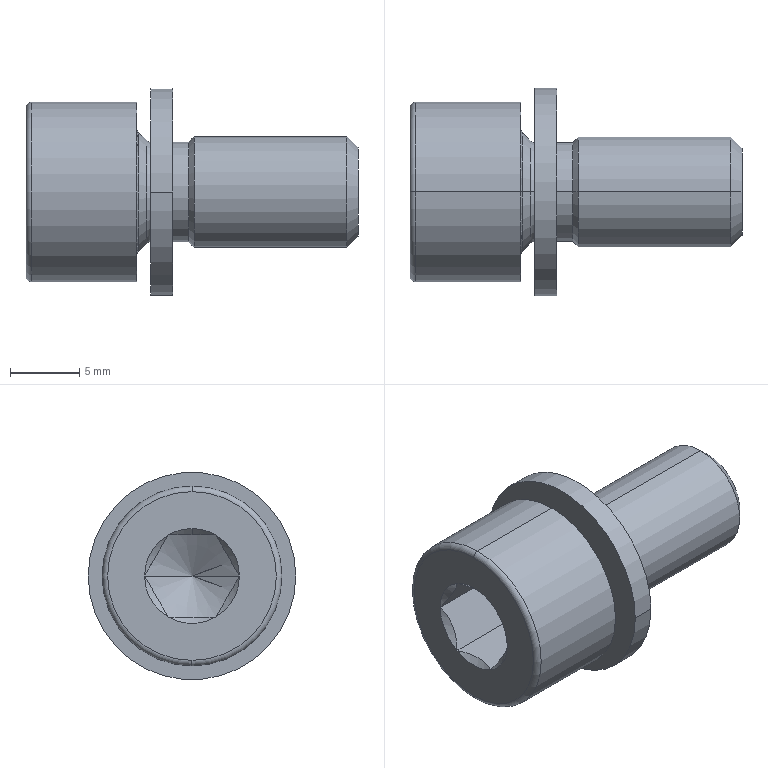Part | SolidWorks | features RevCut 2, Revolution 2, Chamfer 1, Cut 1, Fillet 1 | 2 solids | 48 faces | box 24 x 15 x 15 mm | volume 1870 mm3 | plane 17 | cone 15 | cylinder 10 | torus 6 | commonest cylinder face diameters 7.188 x2 7.55 x2 8 x2 13 x2 15 x2
STEP:
#1=CARTESIAN_POINT('',(10.62,-7.5,0.));
#2=VERTEX_POINT('',#1);
#3=CARTESIAN_POINT('',(10.62,7.5,0.));
#4=VERTEX_POINT('',#3);
#5=CARTESIAN_POINT('',(10.62,0.,0.));
#6=DIRECTION('',(-1.,0.,0.));
#7=DIRECTION('',(0.,-1.,0.));
#8=AXIS2_PLACEMENT_3D('',#5,#6,#7);
#9=CIRCLE('',#8,7.5);
#10=EDGE_CURVE('',#2,#4,#9,.T.);
#11=ORIENTED_EDGE('',*,*,#10,.T.);
#12=CARTESIAN_POINT('',(9.02,7.5,0.));
#13=VERTEX_POINT('',#12);
#14=CARTESIAN_POINT('',(0.,7.5,0.));
#15=DIRECTION('',(-1.,0.,0.));
#16=VECTOR('',#15,1000.);
#17=LINE('',#14,#16);
#18=EDGE_CURVE('',#4,#13,#17,.T.);
#19=ORIENTED_EDGE('',*,*,#18,.T.);
#20=CARTESIAN_POINT('',(9.02,-7.5,0.));
#21=VERTEX_POINT('',#20);
#22=CARTESIAN_POINT('',(9.02,0.,0.));
#23=DIRECTION('',(-1.,0.,0.));
#24=DIRECTION('',(0.,-1.,0.));
#25=AXIS2_PLACEMENT_3D('',#22,#23,#24);
#26=CIRCLE('',#25,7.5);
#27=EDGE_CURVE('',#21,#13,#26,.T.);
#28=ORIENTED_EDGE('',*,*,#27,.F.);
#29=CARTESIAN_POINT('',(0.,-7.5,0.));
#30=DIRECTION('',(-1.,0.,0.));
#31=VECTOR('',#30,1000.);
#32=LINE('',#29,#31);
#33=EDGE_CURVE('',#2,#21,#32,.T.);
#34=ORIENTED_EDGE('',*,*,#33,.F.);
#35=EDGE_LOOP('',(#11,#19,#28,#34));
#36=FACE_OUTER_BOUND('',#35,.T.);
#37=CARTESIAN_POINT('',(0.,0.,0.));
#38=DIRECTION('',(-1.,0.,0.));
#39=DIRECTION('',(0.,-1.,0.));
#40=AXIS2_PLACEMENT_3D('',#37,#38,#39);
#41=CYLINDRICAL_SURFACE('',#40,7.5);
#42=ADVANCED_FACE('',(#36),#41,.T.);
#43=CARTESIAN_POINT('',(10.62,3.775,0.));
#44=VERTEX_POINT('',#43);
#45=CARTESIAN_POINT('',(10.62,-3.775,0.));
#46=VERTEX_POINT('',#45);
#47=CARTESIAN_POINT('',(10.62,0.,0.));
#48=DIRECTION('',(-1.,0.,0.));
#49=DIRECTION('',(0.,-1.,0.));
#50=AXIS2_PLACEMENT_3D('',#47,#48,#49);
#51=CIRCLE('',#50,3.775);
#52=EDGE_CURVE('',#44,#46,#51,.T.);
#53=ORIENTED_EDGE('',*,*,#52,.F.);
#54=CARTESIAN_POINT('',(9.02,3.775,0.));
#55=VERTEX_POINT('',#54);
#56=CARTESIAN_POINT('',(0.,3.775,0.));
#57=DIRECTION('',(-1.,0.,0.));
#58=VECTOR('',#57,1000.);
#59=LINE('',#56,#58);
#60=EDGE_CURVE('',#44,#55,#59,.T.);
#61=ORIENTED_EDGE('',*,*,#60,.T.);
#62=CARTESIAN_POINT('',(9.02,-3.775,0.));
#63=VERTEX_POINT('',#62);
#64=CARTESIAN_POINT('',(9.02,0.,0.));
#65=DIRECTION('',(-1.,0.,0.));
#66=DIRECTION('',(0.,-1.,0.));
#67=AXIS2_PLACEMENT_3D('',#64,#65,#66);
#68=CIRCLE('',#67,3.775);
#69=EDGE_CURVE('',#55,#63,#68,.T.);
#70=ORIENTED_EDGE('',*,*,#69,.T.);
#71=CARTESIAN_POINT('',(0.,-3.775,0.));
#72=DIRECTION('',(-1.,0.,0.));
#73=VECTOR('',#72,1000.);
#74=LINE('',#71,#73);
#75=EDGE_CURVE('',#46,#63,#74,.T.);
#76=ORIENTED_EDGE('',*,*,#75,.F.);
#77=EDGE_LOOP('',(#53,#61,#70,#76));
#78=FACE_OUTER_BOUND('',#77,.T.);
#79=CARTESIAN_POINT('',(0.,0.,0.));
#80=DIRECTION('',(-1.,0.,0.));
#81=DIRECTION('',(0.,-1.,0.));
#82=AXIS2_PLACEMENT_3D('',#79,#80,#81);
#83=CYLINDRICAL_SURFACE('',#82,3.775);
#84=ADVANCED_FACE('',(#78),#83,.F.);
#85=ORIENTED_EDGE('',*,*,#60,.F.);
#86=CARTESIAN_POINT('',(10.62,0.,0.));
#87=DIRECTION('',(-1.,0.,0.));
#88=DIRECTION('',(0.,-1.,0.));
#89=AXIS2_PLACEMENT_3D('',#86,#87,#88);
#90=CIRCLE('',#89,3.775);
#91=EDGE_CURVE('',#46,#44,#90,.T.);
#92=ORIENTED_EDGE('',*,*,#91,.F.);
#93=ORIENTED_EDGE('',*,*,#75,.T.);
#94=CARTESIAN_POINT('',(9.02,0.,0.));
#95=DIRECTION('',(-1.,0.,0.));
#96=DIRECTION('',(0.,-1.,0.));
#97=AXIS2_PLACEMENT_3D('',#94,#95,#96);
#98=CIRCLE('',#97,3.775);
#99=EDGE_CURVE('',#63,#55,#98,.T.);
#100=ORIENTED_EDGE('',*,*,#99,.T.);
#101=EDGE_LOOP('',(#85,#92,#93,#100));
#102=FACE_OUTER_BOUND('',#101,.T.);
#103=CARTESIAN_POINT('',(0.,0.,0.));
#104=DIRECTION('',(-1.,0.,0.));
#105=DIRECTION('',(0.,-1.,0.));
#106=AXIS2_PLACEMENT_3D('',#103,#104,#105);
#107=CYLINDRICAL_SURFACE('',#106,3.775);
#108=ADVANCED_FACE('',(#102),#107,.F.);
#109=ORIENTED_EDGE('',*,*,#99,.F.);
#110=ORIENTED_EDGE('',*,*,#69,.F.);
#111=EDGE_LOOP('',(#109,#110));
#112=FACE_BOUND('',#111,.T.);
#113=ORIENTED_EDGE('',*,*,#27,.T.);
#114=CARTESIAN_POINT('',(9.02,0.,0.));
#115=DIRECTION('',(-1.,0.,0.));
#116=DIRECTION('',(0.,-1.,0.));
#117=AXIS2_PLACEMENT_3D('',#114,#115,#116);
#118=CIRCLE('',#117,7.5);
#119=EDGE_CURVE('',#13,#21,#118,.T.);
#120=ORIENTED_EDGE('',*,*,#119,.T.);
#121=EDGE_LOOP('',(#113,#120));
#122=FACE_OUTER_BOUND('',#121,.T.);
#123=CARTESIAN_POINT('',(9.02,-3.775,0.));
#124=DIRECTION('',(1.,0.,0.));
#125=DIRECTION('',(0.,1.,0.));
#126=AXIS2_PLACEMENT_3D('',#123,#124,#125);
#127=PLANE('',#126);
#128=ADVANCED_FACE('',(#112,#122),#127,.F.);
#129=ORIENTED_EDGE('',*,*,#18,.F.);
#130=CARTESIAN_POINT('',(10.62,0.,0.));
#131=DIRECTION('',(-1.,0.,0.));
#132=DIRECTION('',(0.,-1.,0.));
#133=AXIS2_PLACEMENT_3D('',#130,#131,#132);
#134=CIRCLE('',#133,7.5);
#135=EDGE_CURVE('',#4,#2,#134,.T.);
#136=ORIENTED_EDGE('',*,*,#135,.T.);
#137=ORIENTED_EDGE('',*,*,#33,.T.);
#138=ORIENTED_EDGE('',*,*,#119,.F.);
#139=EDGE_LOOP('',(#129,#136,#137,#138));
#140=FACE_OUTER_BOUND('',#139,.T.);
#141=CARTESIAN_POINT('',(0.,0.,0.));
#142=DIRECTION('',(-1.,0.,0.));
#143=DIRECTION('',(0.,-1.,0.));
#144=AXIS2_PLACEMENT_3D('',#141,#142,#143);
#145=CYLINDRICAL_SURFACE('',#144,7.5);
#146=ADVANCED_FACE('',(#140),#145,.T.);
#147=ORIENTED_EDGE('',*,*,#10,.F.);
#148=ORIENTED_EDGE('',*,*,#135,.F.);
#149=EDGE_LOOP('',(#147,#148));
#150=FACE_OUTER_BOUND('',#149,.T.);
#151=ORIENTED_EDGE('',*,*,#91,.T.);
#152=ORIENTED_EDGE('',*,*,#52,.T.);
#153=EDGE_LOOP('',(#151,#152));
#154=FACE_BOUND('',#153,.T.);
#155=CARTESIAN_POINT('',(10.62,-7.5,0.));
#156=DIRECTION('',(-1.,0.,0.));
#157=DIRECTION('',(0.,-1.,0.));
#158=AXIS2_PLACEMENT_3D('',#155,#156,#157);
#159=PLANE('',#158);
#160=ADVANCED_FACE('',(#150,#154),#159,.F.);
#161=CLOSED_SHELL('',(#42,#84,#108,#128,#146,#160));
#162=MANIFOLD_SOLID_BREP('',#161);
#163=CARTESIAN_POINT('',(24.,0.,-3.2));
#164=VERTEX_POINT('',#163);
#165=CARTESIAN_POINT('',(24.,0.,3.2));
#166=VERTEX_POINT('',#165);
#167=CARTESIAN_POINT('',(24.,0.,0.));
#168=DIRECTION('',(1.,0.,0.));
#169=DIRECTION('',(0.,0.,-1.));
#170=AXIS2_PLACEMENT_3D('',#167,#168,#169);
#171=CIRCLE('',#170,3.2);
#172=EDGE_CURVE('',#164,#166,#171,.T.);
#173=ORIENTED_EDGE('',*,*,#172,.F.);
#174=CARTESIAN_POINT('',(23.2,0.,-4.));
#175=VERTEX_POINT('',#174);
#176=CARTESIAN_POINT('',(24.,0.,-3.2));
#177=DIRECTION('',(-0.7071,0.,-0.7071));
#178=VECTOR('',#177,1000.);
#179=LINE('',#176,#178);
#180=EDGE_CURVE('',#164,#175,#179,.T.);
#181=ORIENTED_EDGE('',*,*,#180,.T.);
#182=CARTESIAN_POINT('',(23.2,0.,4.));
#183=VERTEX_POINT('',#182);
#184=CARTESIAN_POINT('',(23.2,0.,0.));
#185=DIRECTION('',(-1.,0.,0.));
#186=DIRECTION('',(0.,0.,-1.));
#187=AXIS2_PLACEMENT_3D('',#184,#185,#186);
#188=CIRCLE('',#187,4.);
#189=EDGE_CURVE('',#183,#175,#188,.T.);
#190=ORIENTED_EDGE('',*,*,#189,.F.);
#191=CARTESIAN_POINT('',(24.,0.,3.2));
#192=DIRECTION('',(-0.7071,0.,0.7071));
#193=VECTOR('',#192,1000.);
#194=LINE('',#191,#193);
#195=EDGE_CURVE('',#166,#183,#194,.T.);
#196=ORIENTED_EDGE('',*,*,#195,.F.);
#197=EDGE_LOOP('',(#173,#181,#190,#196));
#198=FACE_OUTER_BOUND('',#197,.T.);
#199=CARTESIAN_POINT('',(24.,0.,0.));
#200=DIRECTION('',(-1.,0.,0.));
#201=DIRECTION('',(0.,0.,1.));
#202=AXIS2_PLACEMENT_3D('',#199,#200,#201);
#203=CONICAL_SURFACE('',#202,3.2,0.7854);
#204=ADVANCED_FACE('',(#198),#203,.T.);
#205=CARTESIAN_POINT('',(0.4,0.,-6.5));
#206=VERTEX_POINT('',#205);
#207=CARTESIAN_POINT('',(0.4,0.,6.5));
#208=VERTEX_POINT('',#207);
#209=CARTESIAN_POINT('',(0.4,0.,0.));
#210=DIRECTION('',(1.,0.,0.));
#211=DIRECTION('',(0.,0.,1.));
#212=AXIS2_PLACEMENT_3D('',#209,#210,#211);
#213=CIRCLE('',#212,6.5);
#214=EDGE_CURVE('',#206,#208,#213,.T.);
#215=ORIENTED_EDGE('',*,*,#214,.F.);
#216=CARTESIAN_POINT('',(0.,0.,-6.1));
#217=VERTEX_POINT('',#216);
#218=CARTESIAN_POINT('',(0.4,0.,-6.1));
#219=DIRECTION('',(0.,1.,0.));
#220=DIRECTION('',(0.,0.,1.));
#221=AXIS2_PLACEMENT_3D('',#218,#219,#220);
#222=CIRCLE('',#221,0.4);
#223=EDGE_CURVE('',#206,#217,#222,.T.);
#224=ORIENTED_EDGE('',*,*,#223,.T.);
#225=CARTESIAN_POINT('',(0.,0.,6.1));
#226=VERTEX_POINT('',#225);
#227=CARTESIAN_POINT('',(0.,0.,0.));
#228=DIRECTION('',(-1.,0.,0.));
#229=DIRECTION('',(0.,0.,1.));
#230=AXIS2_PLACEMENT_3D('',#227,#228,#229);
#231=CIRCLE('',#230,6.1);
#232=EDGE_CURVE('',#226,#217,#231,.T.);
#233=ORIENTED_EDGE('',*,*,#232,.F.);
#234=CARTESIAN_POINT('',(0.4,0.,6.1));
#235=DIRECTION('',(0.,-1.,0.));
#236=DIRECTION('',(0.,0.,-1.));
#237=AXIS2_PLACEMENT_3D('',#234,#235,#236);
#238=CIRCLE('',#237,0.4);
#239=EDGE_CURVE('',#208,#226,#238,.T.);
#240=ORIENTED_EDGE('',*,*,#239,.F.);
#241=EDGE_LOOP('',(#215,#224,#233,#240));
#242=FACE_OUTER_BOUND('',#241,.T.);
#243=CARTESIAN_POINT('',(0.4,0.,0.));
#244=DIRECTION('',(-1.,0.,0.));
#245=DIRECTION('',(0.,0.,1.));
#246=AXIS2_PLACEMENT_3D('',#243,#244,#245);
#247=TOROIDAL_SURFACE('',#246,6.1,0.4);
#248=ADVANCED_FACE('',(#242),#247,.T.);
#249=CARTESIAN_POINT('',(6.68,0.,0.));
#250=VERTEX_POINT('',#249);
#251=CARTESIAN_POINT('',(4.7,-3.43,0.));
#252=VERTEX_POINT('',#251);
#253=CARTESIAN_POINT('',(6.68,0.,0.));
#254=DIRECTION('',(-0.5,-0.866,0.));
#255=VECTOR('',#254,1000.);
#256=LINE('',#253,#255);
#257=EDGE_CURVE('',#250,#252,#256,.T.);
#258=ORIENTED_EDGE('',*,*,#257,.F.);
#259=CARTESIAN_POINT('',(4.7,3.43,0.));
#260=VERTEX_POINT('',#259);
#261=CARTESIAN_POINT('',(6.68,0.,0.));
#262=DIRECTION('',(-0.5,0.866,0.));
#263=VECTOR('',#262,1000.);
#264=LINE('',#261,#263);
#265=EDGE_CURVE('',#250,#260,#264,.T.);
#266=ORIENTED_EDGE('',*,*,#265,.T.);
#267=CARTESIAN_POINT('',(4.7,1.715,-2.97));
#268=VERTEX_POINT('',#267);
#269=CARTESIAN_POINT('',(4.7,0.,0.));
#270=DIRECTION('',(-1.,0.,0.));
#271=DIRECTION('',(0.,-1.,0.));
#272=AXIS2_PLACEMENT_3D('',#269,#270,#271);
#273=CIRCLE('',#272,3.43);
#274=EDGE_CURVE('',#260,#268,#273,.T.);
#275=ORIENTED_EDGE('',*,*,#274,.T.);
#276=CARTESIAN_POINT('',(4.7,-1.715,-2.97));
#277=VERTEX_POINT('',#276);
#278=CARTESIAN_POINT('',(4.7,0.,0.));
#279=DIRECTION('',(-1.,0.,0.));
#280=DIRECTION('',(0.,-1.,0.));
#281=AXIS2_PLACEMENT_3D('',#278,#279,#280);
#282=CIRCLE('',#281,3.43);
#283=EDGE_CURVE('',#268,#277,#282,.T.);
#284=ORIENTED_EDGE('',*,*,#283,.T.);
#285=CARTESIAN_POINT('',(4.7,0.,0.));
#286=DIRECTION('',(-1.,0.,0.));
#287=DIRECTION('',(0.,-1.,0.));
#288=AXIS2_PLACEMENT_3D('',#285,#286,#287);
#289=CIRCLE('',#288,3.43);
#290=EDGE_CURVE('',#277,#252,#289,.T.);
#291=ORIENTED_EDGE('',*,*,#290,.T.);
#292=EDGE_LOOP('',(#258,#266,#275,#284,#291));
#293=FACE_OUTER_BOUND('',#292,.T.);
#294=CARTESIAN_POINT('',(-993.32,0.,0.));
#295=DIRECTION('',(-1.,0.,0.));
#296=DIRECTION('',(0.,-1.,0.));
#297=AXIS2_PLACEMENT_3D('',#294,#295,#296);
#298=CONICAL_SURFACE('',#297,1732.051,1.047);
#299=ADVANCED_FACE('',(#293),#298,.F.);
#300=CARTESIAN_POINT('',(0.4595,0.,2.97));
#301=VERTEX_POINT('',#300);
#302=CARTESIAN_POINT('',(0.,1.715,2.97));
#303=VERTEX_POINT('',#302);
#304=CARTESIAN_POINT('',(0.4595,0.,2.97));
#305=CARTESIAN_POINT('',(0.4595,0.3016,2.97));
#306=CARTESIAN_POINT('',(0.4131,0.5952,2.97));
#307=CARTESIAN_POINT('',(0.2902,1.027,2.97));
#308=CARTESIAN_POINT('',(0.2401,1.169,2.97));
#309=CARTESIAN_POINT('',(0.1283,1.447,2.97));
#310=CARTESIAN_POINT('',(0.06637,1.582,2.97));
#311=CARTESIAN_POINT('',(0.,1.715,2.97));
#312=B_SPLINE_CURVE_WITH_KNOTS('',3,(#304,#305,#306,#307,#308,#309,#310,#311),.UNSPECIFIED.,.F.,.F.,(4,2,2,4),(0.004005,0.004894,0.005339,0.005784),.UNSPECIFIED.);
#313=EDGE_CURVE('',#301,#303,#312,.T.);
#314=ORIENTED_EDGE('',*,*,#313,.F.);
#315=CARTESIAN_POINT('',(0.,0.,3.43));
#316=VERTEX_POINT('',#315);
#317=CARTESIAN_POINT('',(0.4595,0.,2.97));
#318=DIRECTION('',(-0.7071,0.,0.7071));
#319=VECTOR('',#318,1000.);
#320=LINE('',#317,#319);
#321=EDGE_CURVE('',#301,#316,#320,.T.);
#322=ORIENTED_EDGE('',*,*,#321,.T.);
#323=CARTESIAN_POINT('',(0.,0.,0.));
#324=DIRECTION('',(1.,0.,0.));
#325=DIRECTION('',(0.,0.,-1.));
#326=AXIS2_PLACEMENT_3D('',#323,#324,#325);
#327=CIRCLE('',#326,3.43);
#328=EDGE_CURVE('',#303,#316,#327,.T.);
#329=ORIENTED_EDGE('',*,*,#328,.F.);
#330=EDGE_LOOP('',(#314,#322,#329));
#331=FACE_OUTER_BOUND('',#330,.T.);
#332=CARTESIAN_POINT('',(0.4595,0.,0.));
#333=DIRECTION('',(-1.,0.,0.));
#334=DIRECTION('',(0.,0.,1.));
#335=AXIS2_PLACEMENT_3D('',#332,#333,#334);
#336=CONICAL_SURFACE('',#335,2.97,0.7854);
#337=ADVANCED_FACE('',(#331),#336,.F.);
#338=CARTESIAN_POINT('',(12.156,0.,-4.));
#339=VERTEX_POINT('',#338);
#340=CARTESIAN_POINT('',(12.156,0.,4.));
#341=VERTEX_POINT('',#340);
#342=CARTESIAN_POINT('',(12.156,0.,0.));
#343=DIRECTION('',(1.,0.,0.));
#344=DIRECTION('',(0.,0.,-1.));
#345=AXIS2_PLACEMENT_3D('',#342,#343,#344);
#346=CIRCLE('',#345,4.);
#347=EDGE_CURVE('',#339,#341,#346,.T.);
#348=ORIENTED_EDGE('',*,*,#347,.T.);
#349=CARTESIAN_POINT('',(0.,0.,4.));
#350=DIRECTION('',(1.,0.,0.));
#351=VECTOR('',#350,1000.);
#352=LINE('',#349,#351);
#353=EDGE_CURVE('',#341,#183,#352,.T.);
#354=ORIENTED_EDGE('',*,*,#353,.T.);
#355=ORIENTED_EDGE('',*,*,#189,.T.);
#356=CARTESIAN_POINT('',(0.,0.,-4.));
#357=DIRECTION('',(1.,0.,0.));
#358=VECTOR('',#357,1000.);
#359=LINE('',#356,#358);
#360=EDGE_CURVE('',#339,#175,#359,.T.);
#361=ORIENTED_EDGE('',*,*,#360,.F.);
#362=EDGE_LOOP('',(#348,#354,#355,#361));
#363=FACE_OUTER_BOUND('',#362,.T.);
#364=CARTESIAN_POINT('',(0.,0.,0.));
#365=DIRECTION('',(1.,0.,0.));
#366=DIRECTION('',(0.,0.,-1.));
#367=AXIS2_PLACEMENT_3D('',#364,#365,#366);
#368=CYLINDRICAL_SURFACE('',#367,4.);
#369=ADVANCED_FACE('',(#363),#368,.T.);
#370=CARTESIAN_POINT('',(11.75,0.,-3.594));
#371=VERTEX_POINT('',#370);
#372=CARTESIAN_POINT('',(11.75,0.,3.594));
#373=VERTEX_POINT('',#372);
#374=CARTESIAN_POINT('',(11.75,0.,0.));
#375=DIRECTION('',(1.,0.,0.));
#376=DIRECTION('',(0.,0.,-1.));
#377=AXIS2_PLACEMENT_3D('',#374,#375,#376);
#378=CIRCLE('',#377,3.594);
#379=EDGE_CURVE('',#371,#373,#378,.T.);
#380=ORIENTED_EDGE('',*,*,#379,.T.);
#381=CARTESIAN_POINT('',(12.156,0.,4.));
#382=DIRECTION('',(0.7071,0.,0.7071));
#383=VECTOR('',#382,1000.);
#384=LINE('',#381,#383);
#385=EDGE_CURVE('',#373,#341,#384,.T.);
#386=ORIENTED_EDGE('',*,*,#385,.T.);
#387=ORIENTED_EDGE('',*,*,#347,.F.);
#388=CARTESIAN_POINT('',(12.156,0.,-4.));
#389=DIRECTION('',(0.7071,0.,-0.7071));
#390=VECTOR('',#389,1000.);
#391=LINE('',#388,#390);
#392=EDGE_CURVE('',#371,#339,#391,.T.);
#393=ORIENTED_EDGE('',*,*,#392,.F.);
#394=EDGE_LOOP('',(#380,#386,#387,#393));
#395=FACE_OUTER_BOUND('',#394,.T.);
#396=CARTESIAN_POINT('',(12.156,0.,0.));
#397=DIRECTION('',(1.,0.,0.));
#398=DIRECTION('',(0.,0.,-1.));
#399=AXIS2_PLACEMENT_3D('',#396,#397,#398);
#400=CONICAL_SURFACE('',#399,4.,0.7854);
#401=ADVANCED_FACE('',(#395),#400,.T.);
#402=CARTESIAN_POINT('',(9.02,0.,-3.594));
#403=VERTEX_POINT('',#402);
#404=CARTESIAN_POINT('',(9.02,0.,3.594));
#405=VERTEX_POINT('',#404);
#406=CARTESIAN_POINT('',(9.02,0.,0.));
#407=DIRECTION('',(1.,0.,0.));
#408=DIRECTION('',(0.,0.,-1.));
#409=AXIS2_PLACEMENT_3D('',#406,#407,#408);
#410=CIRCLE('',#409,3.594);
#411=EDGE_CURVE('',#403,#405,#410,.T.);
#412=ORIENTED_EDGE('',*,*,#411,.T.);
#413=CARTESIAN_POINT('',(0.,0.,3.594));
#414=DIRECTION('',(1.,0.,0.));
#415=VECTOR('',#414,1000.);
#416=LINE('',#413,#415);
#417=EDGE_CURVE('',#405,#373,#416,.T.);
#418=ORIENTED_EDGE('',*,*,#417,.T.);
#419=ORIENTED_EDGE('',*,*,#379,.F.);
#420=CARTESIAN_POINT('',(0.,0.,-3.594));
#421=DIRECTION('',(1.,0.,0.));
#422=VECTOR('',#421,1000.);
#423=LINE('',#420,#422);
#424=EDGE_CURVE('',#403,#371,#423,.T.);
#425=ORIENTED_EDGE('',*,*,#424,.F.);
#426=EDGE_LOOP('',(#412,#418,#419,#425));
#427=FACE_OUTER_BOUND('',#426,.T.);
#428=CARTESIAN_POINT('',(0.,0.,0.));
#429=DIRECTION('',(1.,0.,0.));
#430=DIRECTION('',(0.,0.,-1.));
#431=AXIS2_PLACEMENT_3D('',#428,#429,#430);
#432=CYLINDRICAL_SURFACE('',#431,3.594);
#433=ADVANCED_FACE('',(#427),#432,.T.);
#434=CARTESIAN_POINT('',(9.02,0.,0.));
#435=DIRECTION('',(1.,0.,0.));
#436=DIRECTION('',(0.,0.,-1.));
#437=AXIS2_PLACEMENT_3D('',#434,#435,#436);
#438=CIRCLE('',#437,3.594);
#439=EDGE_CURVE('',#405,#403,#438,.T.);
#440=ORIENTED_EDGE('',*,*,#439,.F.);
#441=CARTESIAN_POINT('',(8.74,0.,3.708));
#442=VERTEX_POINT('',#441);
#443=CARTESIAN_POINT('',(9.02,0.,3.994));
#444=DIRECTION('',(0.,1.,0.));
#445=DIRECTION('',(0.,0.,1.));
#446=AXIS2_PLACEMENT_3D('',#443,#444,#445);
#447=CIRCLE('',#446,0.4);
#448=EDGE_CURVE('',#405,#442,#447,.T.);
#449=ORIENTED_EDGE('',*,*,#448,.T.);
#450=CARTESIAN_POINT('',(8.74,0.,-3.708));
#451=VERTEX_POINT('',#450);
#452=CARTESIAN_POINT('',(8.74,0.,0.));
#453=DIRECTION('',(1.,0.,0.));
#454=DIRECTION('',(0.,0.,-1.));
#455=AXIS2_PLACEMENT_3D('',#452,#453,#454);
#456=CIRCLE('',#455,3.708);
#457=EDGE_CURVE('',#442,#451,#456,.T.);
#458=ORIENTED_EDGE('',*,*,#457,.T.);
#459=CARTESIAN_POINT('',(9.02,0.,-3.994));
#460=DIRECTION('',(0.,-1.,0.));
#461=DIRECTION('',(0.,0.,-1.));
#462=AXIS2_PLACEMENT_3D('',#459,#460,#461);
#463=CIRCLE('',#462,0.4);
#464=EDGE_CURVE('',#403,#451,#463,.T.);
#465=ORIENTED_EDGE('',*,*,#464,.F.);
#466=EDGE_LOOP('',(#440,#449,#458,#465));
#467=FACE_OUTER_BOUND('',#466,.T.);
#468=CARTESIAN_POINT('',(9.02,0.,0.));
#469=DIRECTION('',(1.,0.,0.));
#470=DIRECTION('',(0.,0.,-1.));
#471=AXIS2_PLACEMENT_3D('',#468,#469,#470);
#472=TOROIDAL_SURFACE('',#471,3.994,0.4);
#473=ADVANCED_FACE('',(#467),#472,.F.);
#474=CARTESIAN_POINT('',(8.74,0.,0.));
#475=DIRECTION('',(1.,0.,0.));
#476=DIRECTION('',(0.,0.,-1.));
#477=AXIS2_PLACEMENT_3D('',#474,#475,#476);
#478=CIRCLE('',#477,3.708);
#479=EDGE_CURVE('',#451,#442,#478,.T.);
#480=ORIENTED_EDGE('',*,*,#479,.F.);
#481=CARTESIAN_POINT('',(8.12,0.,-4.314));
#482=VERTEX_POINT('',#481);
#483=CARTESIAN_POINT('',(8.74,0.,-3.708));
#484=DIRECTION('',(-0.7151,0.,-0.699));
#485=VECTOR('',#484,1000.);
#486=LINE('',#483,#485);
#487=EDGE_CURVE('',#451,#482,#486,.T.);
#488=ORIENTED_EDGE('',*,*,#487,.T.);
#489=CARTESIAN_POINT('',(8.12,0.,4.314));
#490=VERTEX_POINT('',#489);
#491=CARTESIAN_POINT('',(8.12,0.,0.));
#492=DIRECTION('',(1.,0.,0.));
#493=DIRECTION('',(0.,0.,-1.));
#494=AXIS2_PLACEMENT_3D('',#491,#492,#493);
#495=CIRCLE('',#494,4.314);
#496=EDGE_CURVE('',#482,#490,#495,.T.);
#497=ORIENTED_EDGE('',*,*,#496,.T.);
#498=CARTESIAN_POINT('',(8.74,0.,3.708));
#499=DIRECTION('',(-0.7151,0.,0.699));
#500=VECTOR('',#499,1000.);
#501=LINE('',#498,#500);
#502=EDGE_CURVE('',#442,#490,#501,.T.);
#503=ORIENTED_EDGE('',*,*,#502,.F.);
#504=EDGE_LOOP('',(#480,#488,#497,#503));
#505=FACE_OUTER_BOUND('',#504,.T.);
#506=CARTESIAN_POINT('',(8.74,0.,0.));
#507=DIRECTION('',(-1.,0.,0.));
#508=DIRECTION('',(0.,0.,1.));
#509=AXIS2_PLACEMENT_3D('',#506,#507,#508);
#510=CONICAL_SURFACE('',#509,3.708,0.774);
#511=ADVANCED_FACE('',(#505),#510,.T.);
#512=CARTESIAN_POINT('',(8.12,0.,0.));
#513=DIRECTION('',(1.,0.,0.));
#514=DIRECTION('',(0.,0.,-1.));
#515=AXIS2_PLACEMENT_3D('',#512,#513,#514);
#516=CIRCLE('',#515,4.314);
#517=EDGE_CURVE('',#490,#482,#516,.T.);
#518=ORIENTED_EDGE('',*,*,#517,.F.);
#519=CARTESIAN_POINT('',(8.,0.,4.6));
#520=VERTEX_POINT('',#519);
#521=CARTESIAN_POINT('',(8.4,0.,4.6));
#522=DIRECTION('',(0.,1.,0.));
#523=DIRECTION('',(0.,0.,1.));
#524=AXIS2_PLACEMENT_3D('',#521,#522,#523);
#525=CIRCLE('',#524,0.4);
#526=EDGE_CURVE('',#490,#520,#525,.T.);
#527=ORIENTED_EDGE('',*,*,#526,.T.);
#528=CARTESIAN_POINT('',(8.,0.,-4.6));
#529=VERTEX_POINT('',#528);
#530=CARTESIAN_POINT('',(8.,0.,0.));
#531=DIRECTION('',(1.,0.,0.));
#532=DIRECTION('',(0.,0.,-1.));
#533=AXIS2_PLACEMENT_3D('',#530,#531,#532);
#534=CIRCLE('',#533,4.6);
#535=EDGE_CURVE('',#520,#529,#534,.T.);
#536=ORIENTED_EDGE('',*,*,#535,.T.);
#537=CARTESIAN_POINT('',(8.4,0.,-4.6));
#538=DIRECTION('',(0.,-1.,0.));
#539=DIRECTION('',(0.,0.,-1.));
#540=AXIS2_PLACEMENT_3D('',#537,#538,#539);
#541=CIRCLE('',#540,0.4);
#542=EDGE_CURVE('',#482,#529,#541,.T.);
#543=ORIENTED_EDGE('',*,*,#542,.F.);
#544=EDGE_LOOP('',(#518,#527,#536,#543));
#545=FACE_OUTER_BOUND('',#544,.T.);
#546=CARTESIAN_POINT('',(8.4,0.,0.));
#547=DIRECTION('',(1.,0.,0.));
#548=DIRECTION('',(0.,0.,-1.));
#549=AXIS2_PLACEMENT_3D('',#546,#547,#548);
#550=TOROIDAL_SURFACE('',#549,4.6,0.4);
#551=ADVANCED_FACE('',(#545),#550,.F.);
#552=ORIENTED_EDGE('',*,*,#214,.T.);
#553=CARTESIAN_POINT('',(8.,0.,6.5));
#554=VERTEX_POINT('',#553);
#555=CARTESIAN_POINT('',(0.,0.,6.5));
#556=DIRECTION('',(1.,0.,0.));
#557=VECTOR('',#556,1000.);
#558=LINE('',#555,#557);
#559=EDGE_CURVE('',#208,#554,#558,.T.);
#560=ORIENTED_EDGE('',*,*,#559,.T.);
#561=CARTESIAN_POINT('',(8.,0.,-6.5));
#562=VERTEX_POINT('',#561);
#563=CARTESIAN_POINT('',(8.,0.,0.));
#564=DIRECTION('',(1.,0.,0.));
#565=DIRECTION('',(0.,0.,-1.));
#566=AXIS2_PLACEMENT_3D('',#563,#564,#565);
#567=CIRCLE('',#566,6.5);
#568=EDGE_CURVE('',#562,#554,#567,.T.);
#569=ORIENTED_EDGE('',*,*,#568,.F.);
#570=CARTESIAN_POINT('',(0.,0.,-6.5));
#571=DIRECTION('',(1.,0.,0.));
#572=VECTOR('',#571,1000.);
#573=LINE('',#570,#572);
#574=EDGE_CURVE('',#206,#562,#573,.T.);
#575=ORIENTED_EDGE('',*,*,#574,.F.);
#576=EDGE_LOOP('',(#552,#560,#569,#575));
#577=FACE_OUTER_BOUND('',#576,.T.);
#578=CARTESIAN_POINT('',(0.,0.,0.));
#579=DIRECTION('',(1.,0.,0.));
#580=DIRECTION('',(0.,0.,-1.));
#581=AXIS2_PLACEMENT_3D('',#578,#579,#580);
#582=CYLINDRICAL_SURFACE('',#581,6.5);
#583=ADVANCED_FACE('',(#577),#582,.T.);
#584=ORIENTED_EDGE('',*,*,#232,.T.);
#585=CARTESIAN_POINT('',(0.,0.,0.));
#586=DIRECTION('',(-1.,0.,0.));
#587=DIRECTION('',(0.,0.,1.));
#588=AXIS2_PLACEMENT_3D('',#585,#586,#587);
#589=CIRCLE('',#588,6.1);
#590=EDGE_CURVE('',#217,#226,#589,.T.);
#591=ORIENTED_EDGE('',*,*,#590,.T.);
#592=EDGE_LOOP('',(#584,#591));
#593=FACE_OUTER_BOUND('',#592,.T.);
#594=CARTESIAN_POINT('',(0.,3.43,0.));
#595=VERTEX_POINT('',#594);
#596=CARTESIAN_POINT('',(0.,0.,0.));
#597=DIRECTION('',(1.,0.,0.));
#598=DIRECTION('',(0.,0.,-1.));
#599=AXIS2_PLACEMENT_3D('',#596,#597,#598);
#600=CIRCLE('',#599,3.43);
#601=EDGE_CURVE('',#595,#303,#600,.T.);
#602=ORIENTED_EDGE('',*,*,#601,.T.);
#603=ORIENTED_EDGE('',*,*,#328,.T.);
#604=CARTESIAN_POINT('',(0.,-1.715,2.97));
#605=VERTEX_POINT('',#604);
#606=CARTESIAN_POINT('',(0.,0.,0.));
#607=DIRECTION('',(1.,0.,0.));
#608=DIRECTION('',(0.,0.,-1.));
#609=AXIS2_PLACEMENT_3D('',#606,#607,#608);
#610=CIRCLE('',#609,3.43);
#611=EDGE_CURVE('',#316,#605,#610,.T.);
#612=ORIENTED_EDGE('',*,*,#611,.T.);
#613=CARTESIAN_POINT('',(0.,-3.43,0.));
#614=VERTEX_POINT('',#613);
#615=CARTESIAN_POINT('',(0.,0.,0.));
#616=DIRECTION('',(1.,0.,0.));
#617=DIRECTION('',(0.,0.,-1.));
#618=AXIS2_PLACEMENT_3D('',#615,#616,#617);
#619=CIRCLE('',#618,3.43);
#620=EDGE_CURVE('',#605,#614,#619,.T.);
#621=ORIENTED_EDGE('',*,*,#620,.T.);
#622=CARTESIAN_POINT('',(0.,-1.715,-2.97));
#623=VERTEX_POINT('',#622);
#624=CARTESIAN_POINT('',(0.,0.,0.));
#625=DIRECTION('',(1.,0.,0.));
#626=DIRECTION('',(0.,0.,-1.));
#627=AXIS2_PLACEMENT_3D('',#624,#625,#626);
#628=CIRCLE('',#627,3.43);
#629=EDGE_CURVE('',#614,#623,#628,.T.);
#630=ORIENTED_EDGE('',*,*,#629,.T.);
#631=CARTESIAN_POINT('',(0.,1.715,-2.97));
#632=VERTEX_POINT('',#631);
#633=CARTESIAN_POINT('',(0.,0.,0.));
#634=DIRECTION('',(1.,0.,0.));
#635=DIRECTION('',(0.,0.,-1.));
#636=AXIS2_PLACEMENT_3D('',#633,#634,#635);
#637=CIRCLE('',#636,3.43);
#638=EDGE_CURVE('',#623,#632,#637,.T.);
#639=ORIENTED_EDGE('',*,*,#638,.T.);
#640=CARTESIAN_POINT('',(0.,0.,0.));
#641=DIRECTION('',(1.,0.,0.));
#642=DIRECTION('',(0.,0.,-1.));
#643=AXIS2_PLACEMENT_3D('',#640,#641,#642);
#644=CIRCLE('',#643,3.43);
#645=EDGE_CURVE('',#632,#595,#644,.T.);
#646=ORIENTED_EDGE('',*,*,#645,.T.);
#647=EDGE_LOOP('',(#602,#603,#612,#621,#630,#639,#646));
#648=FACE_BOUND('',#647,.T.);
#649=CARTESIAN_POINT('',(0.,0.,0.));
#650=DIRECTION('',(-1.,0.,0.));
#651=DIRECTION('',(0.,0.,1.));
#652=AXIS2_PLACEMENT_3D('',#649,#650,#651);
#653=PLANE('',#652);
#654=ADVANCED_FACE('',(#593,#648),#653,.T.);
#655=ORIENTED_EDGE('',*,*,#559,.F.);
#656=CARTESIAN_POINT('',(0.4,0.,0.));
#657=DIRECTION('',(1.,0.,0.));
#658=DIRECTION('',(0.,0.,1.));
#659=AXIS2_PLACEMENT_3D('',#656,#657,#658);
#660=CIRCLE('',#659,6.5);
#661=EDGE_CURVE('',#208,#206,#660,.T.);
#662=ORIENTED_EDGE('',*,*,#661,.T.);
#663=ORIENTED_EDGE('',*,*,#574,.T.);
#664=CARTESIAN_POINT('',(8.,0.,0.));
#665=DIRECTION('',(1.,0.,0.));
#666=DIRECTION('',(0.,0.,-1.));
#667=AXIS2_PLACEMENT_3D('',#664,#665,#666);
#668=CIRCLE('',#667,6.5);
#669=EDGE_CURVE('',#554,#562,#668,.T.);
#670=ORIENTED_EDGE('',*,*,#669,.F.);
#671=EDGE_LOOP('',(#655,#662,#663,#670));
#672=FACE_OUTER_BOUND('',#671,.T.);
#673=CARTESIAN_POINT('',(0.,0.,0.));
#674=DIRECTION('',(1.,0.,0.));
#675=DIRECTION('',(0.,0.,-1.));
#676=AXIS2_PLACEMENT_3D('',#673,#674,#675);
#677=CYLINDRICAL_SURFACE('',#676,6.5);
#678=ADVANCED_FACE('',(#672),#677,.T.);
#679=ORIENTED_EDGE('',*,*,#568,.T.);
#680=ORIENTED_EDGE('',*,*,#669,.T.);
#681=EDGE_LOOP('',(#679,#680));
#682=FACE_OUTER_BOUND('',#681,.T.);
#683=CARTESIAN_POINT('',(8.,0.,0.));
#684=DIRECTION('',(1.,0.,0.));
#685=DIRECTION('',(0.,0.,-1.));
#686=AXIS2_PLACEMENT_3D('',#683,#684,#685);
#687=CIRCLE('',#686,4.6);
#688=EDGE_CURVE('',#529,#520,#687,.T.);
#689=ORIENTED_EDGE('',*,*,#688,.F.);
#690=ORIENTED_EDGE('',*,*,#535,.F.);
#691=EDGE_LOOP('',(#689,#690));
#692=FACE_BOUND('',#691,.T.);
#693=CARTESIAN_POINT('',(8.,6.5,0.));
#694=DIRECTION('',(1.,0.,0.));
#695=DIRECTION('',(0.,0.,-1.));
#696=AXIS2_PLACEMENT_3D('',#693,#694,#695);
#697=PLANE('',#696);
#698=ADVANCED_FACE('',(#682,#692),#697,.T.);
#699=ORIENTED_EDGE('',*,*,#526,.F.);
#700=ORIENTED_EDGE('',*,*,#496,.F.);
#701=ORIENTED_EDGE('',*,*,#542,.T.);
#702=ORIENTED_EDGE('',*,*,#688,.T.);
#703=EDGE_LOOP('',(#699,#700,#701,#702));
#704=FACE_OUTER_BOUND('',#703,.T.);
#705=CARTESIAN_POINT('',(8.4,0.,0.));
#706=DIRECTION('',(1.,0.,0.));
#707=DIRECTION('',(0.,0.,-1.));
#708=AXIS2_PLACEMENT_3D('',#705,#706,#707);
#709=TOROIDAL_SURFACE('',#708,4.6,0.4);
#710=ADVANCED_FACE('',(#704),#709,.F.);
#711=ORIENTED_EDGE('',*,*,#487,.F.);
#712=ORIENTED_EDGE('',*,*,#457,.F.);
#713=ORIENTED_EDGE('',*,*,#502,.T.);
#714=ORIENTED_EDGE('',*,*,#517,.T.);
#715=EDGE_LOOP('',(#711,#712,#713,#714));
#716=FACE_OUTER_BOUND('',#715,.T.);
#717=CARTESIAN_POINT('',(8.74,0.,0.));
#718=DIRECTION('',(-1.,0.,0.));
#719=DIRECTION('',(0.,0.,1.));
#720=AXIS2_PLACEMENT_3D('',#717,#718,#719);
#721=CONICAL_SURFACE('',#720,3.708,0.774);
#722=ADVANCED_FACE('',(#716),#721,.T.);
#723=ORIENTED_EDGE('',*,*,#448,.F.);
#724=ORIENTED_EDGE('',*,*,#411,.F.);
#725=ORIENTED_EDGE('',*,*,#464,.T.);
#726=ORIENTED_EDGE('',*,*,#479,.T.);
#727=EDGE_LOOP('',(#723,#724,#725,#726));
#728=FACE_OUTER_BOUND('',#727,.T.);
#729=CARTESIAN_POINT('',(9.02,0.,0.));
#730=DIRECTION('',(1.,0.,0.));
#731=DIRECTION('',(0.,0.,-1.));
#732=AXIS2_PLACEMENT_3D('',#729,#730,#731);
#733=TOROIDAL_SURFACE('',#732,3.994,0.4);
#734=ADVANCED_FACE('',(#728),#733,.F.);
#735=ORIENTED_EDGE('',*,*,#417,.F.);
#736=ORIENTED_EDGE('',*,*,#439,.T.);
#737=ORIENTED_EDGE('',*,*,#424,.T.);
#738=CARTESIAN_POINT('',(11.75,0.,0.));
#739=DIRECTION('',(1.,0.,0.));
#740=DIRECTION('',(0.,0.,-1.));
#741=AXIS2_PLACEMENT_3D('',#738,#739,#740);
#742=CIRCLE('',#741,3.594);
#743=EDGE_CURVE('',#373,#371,#742,.T.);
#744=ORIENTED_EDGE('',*,*,#743,.F.);
#745=EDGE_LOOP('',(#735,#736,#737,#744));
#746=FACE_OUTER_BOUND('',#745,.T.);
#747=CARTESIAN_POINT('',(0.,0.,0.));
#748=DIRECTION('',(1.,0.,0.));
#749=DIRECTION('',(0.,0.,-1.));
#750=AXIS2_PLACEMENT_3D('',#747,#748,#749);
#751=CYLINDRICAL_SURFACE('',#750,3.594);
#752=ADVANCED_FACE('',(#746),#751,.T.);
#753=ORIENTED_EDGE('',*,*,#385,.F.);
#754=ORIENTED_EDGE('',*,*,#743,.T.);
#755=ORIENTED_EDGE('',*,*,#392,.T.);
#756=CARTESIAN_POINT('',(12.156,0.,0.));
#757=DIRECTION('',(1.,0.,0.));
#758=DIRECTION('',(0.,0.,-1.));
#759=AXIS2_PLACEMENT_3D('',#756,#757,#758);
#760=CIRCLE('',#759,4.);
#761=EDGE_CURVE('',#341,#339,#760,.T.);
#762=ORIENTED_EDGE('',*,*,#761,.F.);
#763=EDGE_LOOP('',(#753,#754,#755,#762));
#764=FACE_OUTER_BOUND('',#763,.T.);
#765=CARTESIAN_POINT('',(12.156,0.,0.));
#766=DIRECTION('',(1.,0.,0.));
#767=DIRECTION('',(0.,0.,-1.));
#768=AXIS2_PLACEMENT_3D('',#765,#766,#767);
#769=CONICAL_SURFACE('',#768,4.,0.7854);
#770=ADVANCED_FACE('',(#764),#769,.T.);
#771=ORIENTED_EDGE('',*,*,#353,.F.);
#772=ORIENTED_EDGE('',*,*,#761,.T.);
#773=ORIENTED_EDGE('',*,*,#360,.T.);
#774=CARTESIAN_POINT('',(23.2,0.,0.));
#775=DIRECTION('',(-1.,0.,0.));
#776=DIRECTION('',(0.,0.,-1.));
#777=AXIS2_PLACEMENT_3D('',#774,#775,#776);
#778=CIRCLE('',#777,4.);
#779=EDGE_CURVE('',#175,#183,#778,.T.);
#780=ORIENTED_EDGE('',*,*,#779,.T.);
#781=EDGE_LOOP('',(#771,#772,#773,#780));
#782=FACE_OUTER_BOUND('',#781,.T.);
#783=CARTESIAN_POINT('',(0.,0.,0.));
#784=DIRECTION('',(1.,0.,0.));
#785=DIRECTION('',(0.,0.,-1.));
#786=AXIS2_PLACEMENT_3D('',#783,#784,#785);
#787=CYLINDRICAL_SURFACE('',#786,4.);
#788=ADVANCED_FACE('',(#782),#787,.T.);
#789=CARTESIAN_POINT('',(24.,0.,0.));
#790=DIRECTION('',(1.,0.,0.));
#791=DIRECTION('',(0.,0.,-1.));
#792=AXIS2_PLACEMENT_3D('',#789,#790,#791);
#793=CIRCLE('',#792,3.2);
#794=EDGE_CURVE('',#166,#164,#793,.T.);
#795=ORIENTED_EDGE('',*,*,#794,.T.);
#796=ORIENTED_EDGE('',*,*,#172,.T.);
#797=EDGE_LOOP('',(#795,#796));
#798=FACE_OUTER_BOUND('',#797,.T.);
#799=CARTESIAN_POINT('',(24.,4.,0.));
#800=DIRECTION('',(1.,0.,0.));
#801=DIRECTION('',(0.,0.,-1.));
#802=AXIS2_PLACEMENT_3D('',#799,#800,#801);
#803=PLANE('',#802);
#804=ADVANCED_FACE('',(#798),#803,.T.);
#805=ORIENTED_EDGE('',*,*,#321,.F.);
#806=CARTESIAN_POINT('',(0.,-1.715,2.97));
#807=CARTESIAN_POINT('',(0.133,-1.449,2.97));
#808=CARTESIAN_POINT('',(0.2495,-1.169,2.97));
#809=CARTESIAN_POINT('',(0.4126,-0.5969,2.97));
#810=CARTESIAN_POINT('',(0.4595,-0.3013,2.97));
#811=CARTESIAN_POINT('',(0.4595,0.,2.97));
#812=B_SPLINE_CURVE_WITH_KNOTS('',3,(#806,#807,#808,#809,#810,#811),.UNSPECIFIED.,.F.,.F.,(4,2,4),(0.002228,0.003116,0.004005),.UNSPECIFIED.);
#813=EDGE_CURVE('',#605,#301,#812,.T.);
#814=ORIENTED_EDGE('',*,*,#813,.F.);
#815=ORIENTED_EDGE('',*,*,#611,.F.);
#816=EDGE_LOOP('',(#805,#814,#815));
#817=FACE_OUTER_BOUND('',#816,.T.);
#818=CARTESIAN_POINT('',(0.4595,0.,0.));
#819=DIRECTION('',(-1.,0.,0.));
#820=DIRECTION('',(0.,0.,1.));
#821=AXIS2_PLACEMENT_3D('',#818,#819,#820);
#822=CONICAL_SURFACE('',#821,2.97,0.7854);
#823=ADVANCED_FACE('',(#817),#822,.F.);
#824=CARTESIAN_POINT('',(0.,1.715,2.97));
#825=CARTESIAN_POINT('',(0.134,1.849,2.738));
#826=CARTESIAN_POINT('',(0.2479,1.986,2.501));
#827=CARTESIAN_POINT('',(0.37,2.199,2.132));
#828=CARTESIAN_POINT('',(0.4025,2.271,2.007));
#829=CARTESIAN_POINT('',(0.4472,2.419,1.752));
#830=CARTESIAN_POINT('',(0.4592,2.494,1.62));
#831=CARTESIAN_POINT('',(0.4602,2.719,1.231));
#832=CARTESIAN_POINT('',(0.4148,2.866,0.9765));
#833=CARTESIAN_POINT('',(0.2504,3.156,0.4738));
#834=CARTESIAN_POINT('',(0.1348,3.295,0.2335));
#835=CARTESIAN_POINT('',(0.,3.43,0.));
#836=B_SPLINE_CURVE_WITH_KNOTS('',3,(#824,#825,#826,#827,#828,#829,#830,#831,#832,#833,#834,#835),.UNSPECIFIED.,.F.,.F.,(4,2,2,2,2,4),(0.000000254,0.000886,0.001329,0.001772,0.002658,0.003543),.UNSPECIFIED.);
#837=EDGE_CURVE('',#303,#595,#836,.T.);
#838=ORIENTED_EDGE('',*,*,#837,.F.);
#839=ORIENTED_EDGE('',*,*,#601,.F.);
#840=EDGE_LOOP('',(#838,#839));
#841=FACE_OUTER_BOUND('',#840,.T.);
#842=CARTESIAN_POINT('',(0.4595,0.,0.));
#843=DIRECTION('',(-1.,0.,0.));
#844=DIRECTION('',(0.,0.,1.));
#845=AXIS2_PLACEMENT_3D('',#842,#843,#844);
#846=CONICAL_SURFACE('',#845,2.97,0.7854);
#847=ADVANCED_FACE('',(#841),#846,.F.);
#848=CARTESIAN_POINT('',(0.,3.43,0.));
#849=CARTESIAN_POINT('',(0.134,3.296,-0.2321));
#850=CARTESIAN_POINT('',(0.2479,3.159,-0.4694));
#851=CARTESIAN_POINT('',(0.37,2.946,-0.8381));
#852=CARTESIAN_POINT('',(0.4025,2.874,-0.9632));
#853=CARTESIAN_POINT('',(0.4472,2.726,-1.219));
#854=CARTESIAN_POINT('',(0.4592,2.651,-1.35));
#855=CARTESIAN_POINT('',(0.4602,2.426,-1.739));
#856=CARTESIAN_POINT('',(0.4148,2.279,-1.994));
#857=CARTESIAN_POINT('',(0.2504,1.989,-2.497));
#858=CARTESIAN_POINT('',(0.1348,1.85,-2.737));
#859=CARTESIAN_POINT('',(0.,1.715,-2.97));
#860=B_SPLINE_CURVE_WITH_KNOTS('',3,(#848,#849,#850,#851,#852,#853,#854,#855,#856,#857,#858,#859),.UNSPECIFIED.,.F.,.F.,(4,2,2,2,2,4),(0.000000254,0.000886,0.001329,0.001772,0.002658,0.003543),.UNSPECIFIED.);
#861=EDGE_CURVE('',#595,#632,#860,.T.);
#862=ORIENTED_EDGE('',*,*,#861,.F.);
#863=ORIENTED_EDGE('',*,*,#645,.F.);
#864=EDGE_LOOP('',(#862,#863));
#865=FACE_OUTER_BOUND('',#864,.T.);
#866=CARTESIAN_POINT('',(0.4595,0.,0.));
#867=DIRECTION('',(-1.,0.,0.));
#868=DIRECTION('',(0.,0.,1.));
#869=AXIS2_PLACEMENT_3D('',#866,#867,#868);
#870=CONICAL_SURFACE('',#869,2.97,0.7854);
#871=ADVANCED_FACE('',(#865),#870,.F.);
#872=ORIENTED_EDGE('',*,*,#638,.F.);
#873=CARTESIAN_POINT('',(0.,1.715,-2.97));
#874=CARTESIAN_POINT('',(0.06633,1.582,-2.97));
#875=CARTESIAN_POINT('',(0.1282,1.447,-2.97));
#876=CARTESIAN_POINT('',(0.24,1.17,-2.97));
#877=CARTESIAN_POINT('',(0.2901,1.027,-2.97));
#878=CARTESIAN_POINT('',(0.4129,0.5958,-2.97));
#879=CARTESIAN_POINT('',(0.4594,0.3023,-2.97));
#880=CARTESIAN_POINT('',(0.4596,-0.3006,-2.97));
#881=CARTESIAN_POINT('',(0.4127,-0.5964,-2.97));
#882=CARTESIAN_POINT('',(0.2496,-1.169,-2.97));
#883=CARTESIAN_POINT('',(0.133,-1.449,-2.97));
#884=CARTESIAN_POINT('',(0.,-1.715,-2.97));
#885=B_SPLINE_CURVE_WITH_KNOTS('',3,(#873,#874,#875,#876,#877,#878,#879,#880,#881,#882,#883,#884),.UNSPECIFIED.,.F.,.F.,(4,2,2,2,2,4),(0.001823,0.002268,0.002712,0.0036,0.004489,0.005377),.UNSPECIFIED.);
#886=EDGE_CURVE('',#632,#623,#885,.T.);
#887=ORIENTED_EDGE('',*,*,#886,.F.);
#888=EDGE_LOOP('',(#872,#887));
#889=FACE_OUTER_BOUND('',#888,.T.);
#890=CARTESIAN_POINT('',(0.4595,0.,0.));
#891=DIRECTION('',(-1.,0.,0.));
#892=DIRECTION('',(0.,0.,1.));
#893=AXIS2_PLACEMENT_3D('',#890,#891,#892);
#894=CONICAL_SURFACE('',#893,2.97,0.7854);
#895=ADVANCED_FACE('',(#889),#894,.F.);
#896=ORIENTED_EDGE('',*,*,#629,.F.);
#897=CARTESIAN_POINT('',(0.,-1.715,-2.97));
#898=CARTESIAN_POINT('',(0.134,-1.849,-2.738));
#899=CARTESIAN_POINT('',(0.2479,-1.986,-2.501));
#900=CARTESIAN_POINT('',(0.37,-2.199,-2.132));
#901=CARTESIAN_POINT('',(0.4025,-2.271,-2.007));
#902=CARTESIAN_POINT('',(0.4472,-2.419,-1.752));
#903=CARTESIAN_POINT('',(0.4592,-2.494,-1.62));
#904=CARTESIAN_POINT('',(0.4602,-2.719,-1.231));
#905=CARTESIAN_POINT('',(0.4148,-2.866,-0.9765));
#906=CARTESIAN_POINT('',(0.2504,-3.156,-0.4738));
#907=CARTESIAN_POINT('',(0.1348,-3.295,-0.2335));
#908=CARTESIAN_POINT('',(0.,-3.43,0.));
#909=B_SPLINE_CURVE_WITH_KNOTS('',3,(#897,#898,#899,#900,#901,#902,#903,#904,#905,#906,#907,#908),.UNSPECIFIED.,.F.,.F.,(4,2,2,2,2,4),(0.000000254,0.000886,0.001329,0.001772,0.002658,0.003543),.UNSPECIFIED.);
#910=EDGE_CURVE('',#623,#614,#909,.T.);
#911=ORIENTED_EDGE('',*,*,#910,.F.);
#912=EDGE_LOOP('',(#896,#911));
#913=FACE_OUTER_BOUND('',#912,.T.);
#914=CARTESIAN_POINT('',(0.4595,0.,0.));
#915=DIRECTION('',(-1.,0.,0.));
#916=DIRECTION('',(0.,0.,1.));
#917=AXIS2_PLACEMENT_3D('',#914,#915,#916);
#918=CONICAL_SURFACE('',#917,2.97,0.7854);
#919=ADVANCED_FACE('',(#913),#918,.F.);
#920=ORIENTED_EDGE('',*,*,#620,.F.);
#921=CARTESIAN_POINT('',(0.,-3.43,0.));
#922=CARTESIAN_POINT('',(0.134,-3.296,0.2321));
#923=CARTESIAN_POINT('',(0.2479,-3.159,0.4694));
#924=CARTESIAN_POINT('',(0.37,-2.946,0.8381));
#925=CARTESIAN_POINT('',(0.4025,-2.874,0.9632));
#926=CARTESIAN_POINT('',(0.4472,-2.726,1.219));
#927=CARTESIAN_POINT('',(0.4592,-2.651,1.35));
#928=CARTESIAN_POINT('',(0.4602,-2.426,1.739));
#929=CARTESIAN_POINT('',(0.4148,-2.279,1.994));
#930=CARTESIAN_POINT('',(0.2504,-1.989,2.497));
#931=CARTESIAN_POINT('',(0.1348,-1.85,2.737));
#932=CARTESIAN_POINT('',(0.,-1.715,2.97));
#933=B_SPLINE_CURVE_WITH_KNOTS('',3,(#921,#922,#923,#924,#925,#926,#927,#928,#929,#930,#931,#932),.UNSPECIFIED.,.F.,.F.,(4,2,2,2,2,4),(0.000000254,0.000886,0.001329,0.001772,0.002658,0.003543),.UNSPECIFIED.);
#934=EDGE_CURVE('',#614,#605,#933,.T.);
#935=ORIENTED_EDGE('',*,*,#934,.F.);
#936=EDGE_LOOP('',(#920,#935));
#937=FACE_OUTER_BOUND('',#936,.T.);
#938=CARTESIAN_POINT('',(0.4595,0.,0.));
#939=DIRECTION('',(-1.,0.,0.));
#940=DIRECTION('',(0.,0.,1.));
#941=AXIS2_PLACEMENT_3D('',#938,#939,#940);
#942=CONICAL_SURFACE('',#941,2.97,0.7854);
#943=ADVANCED_FACE('',(#937),#942,.F.);
#944=CARTESIAN_POINT('',(4.7,-1.715,2.97));
#945=VERTEX_POINT('',#944);
#946=CARTESIAN_POINT('',(4.7,-1.715,2.97));
#947=DIRECTION('',(-1.,0.,0.));
#948=VECTOR('',#947,1000.);
#949=LINE('',#946,#948);
#950=EDGE_CURVE('',#945,#605,#949,.T.);
#951=ORIENTED_EDGE('',*,*,#950,.T.);
#952=ORIENTED_EDGE('',*,*,#813,.T.);
#953=ORIENTED_EDGE('',*,*,#313,.T.);
#954=CARTESIAN_POINT('',(4.7,1.715,2.97));
#955=VERTEX_POINT('',#954);
#956=CARTESIAN_POINT('',(4.7,1.715,2.97));
#957=DIRECTION('',(-1.,0.,0.));
#958=VECTOR('',#957,1000.);
#959=LINE('',#956,#958);
#960=EDGE_CURVE('',#955,#303,#959,.T.);
#961=ORIENTED_EDGE('',*,*,#960,.F.);
#962=CARTESIAN_POINT('',(4.7,-1.715,2.97));
#963=DIRECTION('',(0.,1.,0.));
#964=VECTOR('',#963,1000.);
#965=LINE('',#962,#964);
#966=EDGE_CURVE('',#945,#955,#965,.T.);
#967=ORIENTED_EDGE('',*,*,#966,.F.);
#968=EDGE_LOOP('',(#951,#952,#953,#961,#967));
#969=FACE_OUTER_BOUND('',#968,.T.);
#970=CARTESIAN_POINT('',(4.7,-1.715,2.97));
#971=DIRECTION('',(0.,0.,1.));
#972=DIRECTION('',(0.,-1.,0.));
#973=AXIS2_PLACEMENT_3D('',#970,#971,#972);
#974=PLANE('',#973);
#975=ADVANCED_FACE('',(#969),#974,.F.);
#976=ORIENTED_EDGE('',*,*,#960,.T.);
#977=ORIENTED_EDGE('',*,*,#837,.T.);
#978=CARTESIAN_POINT('',(4.7,3.43,0.));
#979=DIRECTION('',(-1.,0.,0.));
#980=VECTOR('',#979,1000.);
#981=LINE('',#978,#980);
#982=EDGE_CURVE('',#260,#595,#981,.T.);
#983=ORIENTED_EDGE('',*,*,#982,.F.);
#984=CARTESIAN_POINT('',(4.7,1.715,2.97));
#985=DIRECTION('',(0.,0.5,-0.866));
#986=VECTOR('',#985,1000.);
#987=LINE('',#984,#986);
#988=EDGE_CURVE('',#955,#260,#987,.T.);
#989=ORIENTED_EDGE('',*,*,#988,.F.);
#990=EDGE_LOOP('',(#976,#977,#983,#989));
#991=FACE_OUTER_BOUND('',#990,.T.);
#992=CARTESIAN_POINT('',(4.7,1.715,2.97));
#993=DIRECTION('',(0.,0.866,0.5));
#994=DIRECTION('',(0.,-0.5,0.866));
#995=AXIS2_PLACEMENT_3D('',#992,#993,#994);
#996=PLANE('',#995);
#997=ADVANCED_FACE('',(#991),#996,.F.);
#998=ORIENTED_EDGE('',*,*,#982,.T.);
#999=ORIENTED_EDGE('',*,*,#861,.T.);
#1000=CARTESIAN_POINT('',(4.7,1.715,-2.97));
#1001=DIRECTION('',(-1.,0.,0.));
#1002=VECTOR('',#1001,1000.);
#1003=LINE('',#1000,#1002);
#1004=EDGE_CURVE('',#268,#632,#1003,.T.);
#1005=ORIENTED_EDGE('',*,*,#1004,.F.);
#1006=CARTESIAN_POINT('',(4.7,3.43,0.));
#1007=DIRECTION('',(0.,-0.5,-0.866));
#1008=VECTOR('',#1007,1000.);
#1009=LINE('',#1006,#1008);
#1010=EDGE_CURVE('',#260,#268,#1009,.T.);
#1011=ORIENTED_EDGE('',*,*,#1010,.F.);
#1012=EDGE_LOOP('',(#998,#999,#1005,#1011));
#1013=FACE_OUTER_BOUND('',#1012,.T.);
#1014=CARTESIAN_POINT('',(4.7,3.43,0.));
#1015=DIRECTION('',(0.,0.866,-0.5));
#1016=DIRECTION('',(0.,0.5,0.866));
#1017=AXIS2_PLACEMENT_3D('',#1014,#1015,#1016);
#1018=PLANE('',#1017);
#1019=ADVANCED_FACE('',(#1013),#1018,.F.);
#1020=ORIENTED_EDGE('',*,*,#1004,.T.);
#1021=ORIENTED_EDGE('',*,*,#886,.T.);
#1022=CARTESIAN_POINT('',(4.7,-1.715,-2.97));
#1023=DIRECTION('',(-1.,0.,0.));
#1024=VECTOR('',#1023,1000.);
#1025=LINE('',#1022,#1024);
#1026=EDGE_CURVE('',#277,#623,#1025,.T.);
#1027=ORIENTED_EDGE('',*,*,#1026,.F.);
#1028=CARTESIAN_POINT('',(4.7,1.715,-2.97));
#1029=DIRECTION('',(0.,-1.,0.));
#1030=VECTOR('',#1029,1000.);
#1031=LINE('',#1028,#1030);
#1032=EDGE_CURVE('',#268,#277,#1031,.T.);
#1033=ORIENTED_EDGE('',*,*,#1032,.F.);
#1034=EDGE_LOOP('',(#1020,#1021,#1027,#1033));
#1035=FACE_OUTER_BOUND('',#1034,.T.);
#1036=CARTESIAN_POINT('',(4.7,1.715,-2.97));
#1037=DIRECTION('',(0.,0.,-1.));
#1038=DIRECTION('',(0.,1.,0.));
#1039=AXIS2_PLACEMENT_3D('',#1036,#1037,#1038);
#1040=PLANE('',#1039);
#1041=ADVANCED_FACE('',(#1035),#1040,.F.);
#1042=ORIENTED_EDGE('',*,*,#1026,.T.);
#1043=ORIENTED_EDGE('',*,*,#910,.T.);
#1044=CARTESIAN_POINT('',(4.7,-3.43,0.));
#1045=DIRECTION('',(-1.,0.,0.));
#1046=VECTOR('',#1045,1000.);
#1047=LINE('',#1044,#1046);
#1048=EDGE_CURVE('',#252,#614,#1047,.T.);
#1049=ORIENTED_EDGE('',*,*,#1048,.F.);
#1050=CARTESIAN_POINT('',(4.7,-1.715,-2.97));
#1051=DIRECTION('',(0.,-0.5,0.866));
#1052=VECTOR('',#1051,1000.);
#1053=LINE('',#1050,#1052);
#1054=EDGE_CURVE('',#277,#252,#1053,.T.);
#1055=ORIENTED_EDGE('',*,*,#1054,.F.);
#1056=EDGE_LOOP('',(#1042,#1043,#1049,#1055));
#1057=FACE_OUTER_BOUND('',#1056,.T.);
#1058=CARTESIAN_POINT('',(4.7,-1.715,-2.97));
#1059=DIRECTION('',(0.,-0.866,-0.5));
#1060=DIRECTION('',(0.,0.5,-0.866));
#1061=AXIS2_PLACEMENT_3D('',#1058,#1059,#1060);
#1062=PLANE('',#1061);
#1063=ADVANCED_FACE('',(#1057),#1062,.F.);
#1064=ORIENTED_EDGE('',*,*,#1048,.T.);
#1065=ORIENTED_EDGE('',*,*,#934,.T.);
#1066=ORIENTED_EDGE('',*,*,#950,.F.);
#1067=CARTESIAN_POINT('',(4.7,-3.43,0.));
#1068=DIRECTION('',(0.,0.5,0.866));
#1069=VECTOR('',#1068,1000.);
#1070=LINE('',#1067,#1069);
#1071=EDGE_CURVE('',#252,#945,#1070,.T.);
#1072=ORIENTED_EDGE('',*,*,#1071,.F.);
#1073=EDGE_LOOP('',(#1064,#1065,#1066,#1072));
#1074=FACE_OUTER_BOUND('',#1073,.T.);
#1075=CARTESIAN_POINT('',(4.7,-3.43,0.));
#1076=DIRECTION('',(0.,-0.866,0.5));
#1077=DIRECTION('',(0.,-0.5,-0.866));
#1078=AXIS2_PLACEMENT_3D('',#1075,#1076,#1077);
#1079=PLANE('',#1078);
#1080=ADVANCED_FACE('',(#1074),#1079,.F.);
#1081=ORIENTED_EDGE('',*,*,#1071,.T.);
#1082=CARTESIAN_POINT('',(4.7,0.,0.));
#1083=DIRECTION('',(-1.,0.,0.));
#1084=DIRECTION('',(0.,-1.,0.));
#1085=AXIS2_PLACEMENT_3D('',#1082,#1083,#1084);
#1086=CIRCLE('',#1085,3.43);
#1087=EDGE_CURVE('',#252,#945,#1086,.T.);
#1088=ORIENTED_EDGE('',*,*,#1087,.F.);
#1089=EDGE_LOOP('',(#1081,#1088));
#1090=FACE_OUTER_BOUND('',#1089,.T.);
#1091=CARTESIAN_POINT('',(4.7,-3.43,0.));
#1092=DIRECTION('',(1.,0.,0.));
#1093=DIRECTION('',(0.,1.,0.));
#1094=AXIS2_PLACEMENT_3D('',#1091,#1092,#1093);
#1095=PLANE('',#1094);
#1096=ADVANCED_FACE('',(#1090),#1095,.T.);
#1097=ORIENTED_EDGE('',*,*,#966,.T.);
#1098=CARTESIAN_POINT('',(4.7,0.,0.));
#1099=DIRECTION('',(-1.,0.,0.));
#1100=DIRECTION('',(0.,-1.,0.));
#1101=AXIS2_PLACEMENT_3D('',#1098,#1099,#1100);
#1102=CIRCLE('',#1101,3.43);
#1103=EDGE_CURVE('',#945,#955,#1102,.T.);
#1104=ORIENTED_EDGE('',*,*,#1103,.F.);
#1105=EDGE_LOOP('',(#1097,#1104));
#1106=FACE_OUTER_BOUND('',#1105,.T.);
#1107=CARTESIAN_POINT('',(4.7,-3.43,0.));
#1108=DIRECTION('',(1.,0.,0.));
#1109=DIRECTION('',(0.,1.,0.));
#1110=AXIS2_PLACEMENT_3D('',#1107,#1108,#1109);
#1111=PLANE('',#1110);
#1112=ADVANCED_FACE('',(#1106),#1111,.T.);
#1113=ORIENTED_EDGE('',*,*,#988,.T.);
#1114=CARTESIAN_POINT('',(4.7,0.,0.));
#1115=DIRECTION('',(-1.,0.,0.));
#1116=DIRECTION('',(0.,-1.,0.));
#1117=AXIS2_PLACEMENT_3D('',#1114,#1115,#1116);
#1118=CIRCLE('',#1117,3.43);
#1119=EDGE_CURVE('',#955,#260,#1118,.T.);
#1120=ORIENTED_EDGE('',*,*,#1119,.F.);
#1121=EDGE_LOOP('',(#1113,#1120));
#1122=FACE_OUTER_BOUND('',#1121,.T.);
#1123=CARTESIAN_POINT('',(4.7,-3.43,0.));
#1124=DIRECTION('',(1.,0.,0.));
#1125=DIRECTION('',(0.,1.,0.));
#1126=AXIS2_PLACEMENT_3D('',#1123,#1124,#1125);
#1127=PLANE('',#1126);
#1128=ADVANCED_FACE('',(#1122),#1127,.T.);
#1129=ORIENTED_EDGE('',*,*,#1010,.T.);
#1130=ORIENTED_EDGE('',*,*,#274,.F.);
#1131=EDGE_LOOP('',(#1129,#1130));
#1132=FACE_OUTER_BOUND('',#1131,.T.);
#1133=CARTESIAN_POINT('',(4.7,-3.43,0.));
#1134=DIRECTION('',(1.,0.,0.));
#1135=DIRECTION('',(0.,1.,0.));
#1136=AXIS2_PLACEMENT_3D('',#1133,#1134,#1135);
#1137=PLANE('',#1136);
#1138=ADVANCED_FACE('',(#1132),#1137,.T.);
#1139=ORIENTED_EDGE('',*,*,#1032,.T.);
#1140=ORIENTED_EDGE('',*,*,#283,.F.);
#1141=EDGE_LOOP('',(#1139,#1140));
#1142=FACE_OUTER_BOUND('',#1141,.T.);
#1143=CARTESIAN_POINT('',(4.7,-3.43,0.));
#1144=DIRECTION('',(1.,0.,0.));
#1145=DIRECTION('',(0.,1.,0.));
#1146=AXIS2_PLACEMENT_3D('',#1143,#1144,#1145);
#1147=PLANE('',#1146);
#1148=ADVANCED_FACE('',(#1142),#1147,.T.);
#1149=ORIENTED_EDGE('',*,*,#1054,.T.);
#1150=ORIENTED_EDGE('',*,*,#290,.F.);
#1151=EDGE_LOOP('',(#1149,#1150));
#1152=FACE_OUTER_BOUND('',#1151,.T.);
#1153=CARTESIAN_POINT('',(4.7,-3.43,0.));
#1154=DIRECTION('',(1.,0.,0.));
#1155=DIRECTION('',(0.,1.,0.));
#1156=AXIS2_PLACEMENT_3D('',#1153,#1154,#1155);
#1157=PLANE('',#1156);
#1158=ADVANCED_FACE('',(#1152),#1157,.T.);
#1159=ORIENTED_EDGE('',*,*,#265,.F.);
#1160=ORIENTED_EDGE('',*,*,#257,.T.);
#1161=ORIENTED_EDGE('',*,*,#1087,.T.);
#1162=ORIENTED_EDGE('',*,*,#1103,.T.);
#1163=ORIENTED_EDGE('',*,*,#1119,.T.);
#1164=EDGE_LOOP('',(#1159,#1160,#1161,#1162,#1163));
#1165=FACE_OUTER_BOUND('',#1164,.T.);
#1166=CARTESIAN_POINT('',(-993.32,0.,0.));
#1167=DIRECTION('',(-1.,0.,0.));
#1168=DIRECTION('',(0.,-1.,0.));
#1169=AXIS2_PLACEMENT_3D('',#1166,#1167,#1168);
#1170=CONICAL_SURFACE('',#1169,1732.051,1.047);
#1171=ADVANCED_FACE('',(#1165),#1170,.F.);
#1172=ORIENTED_EDGE('',*,*,#223,.F.);
#1173=ORIENTED_EDGE('',*,*,#661,.F.);
#1174=ORIENTED_EDGE('',*,*,#239,.T.);
#1175=ORIENTED_EDGE('',*,*,#590,.F.);
#1176=EDGE_LOOP('',(#1172,#1173,#1174,#1175));
#1177=FACE_OUTER_BOUND('',#1176,.T.);
#1178=CARTESIAN_POINT('',(0.4,0.,0.));
#1179=DIRECTION('',(-1.,0.,0.));
#1180=DIRECTION('',(0.,0.,1.));
#1181=AXIS2_PLACEMENT_3D('',#1178,#1179,#1180);
#1182=TOROIDAL_SURFACE('',#1181,6.1,0.4);
#1183=ADVANCED_FACE('',(#1177),#1182,.T.);
#1184=ORIENTED_EDGE('',*,*,#180,.F.);
#1185=ORIENTED_EDGE('',*,*,#794,.F.);
#1186=ORIENTED_EDGE('',*,*,#195,.T.);
#1187=ORIENTED_EDGE('',*,*,#779,.F.);
#1188=EDGE_LOOP('',(#1184,#1185,#1186,#1187));
#1189=FACE_OUTER_BOUND('',#1188,.T.);
#1190=CARTESIAN_POINT('',(24.,0.,0.));
#1191=DIRECTION('',(-1.,0.,0.));
#1192=DIRECTION('',(0.,0.,1.));
#1193=AXIS2_PLACEMENT_3D('',#1190,#1191,#1192);
#1194=CONICAL_SURFACE('',#1193,3.2,0.7854);
#1195=ADVANCED_FACE('',(#1189),#1194,.T.);
#1196=CLOSED_SHELL('',(#204,#248,#299,#337,#369,#401,#433,#473,#511,#551,#583,#654,#678,#698,#710,#722,#734,#752,#770,#788,#804,#823,#847,#871,#895,#919,#943,#975,#997,#1019,#1041,#1063,#1080,#1096,#1112,#1128,#1138,#1148,#1158,#1171,#1183,#1195));
#1197=MANIFOLD_SOLID_BREP('',#1196);
#1198=CARTESIAN_POINT('',(0.,0.,0.));
#1199=DIRECTION('',(0.,0.,1.));
#1200=DIRECTION('',(1.,0.,0.));
#1201=AXIS2_PLACEMENT_3D('',#1198,#1199,#1200);
#1202=(LENGTH_UNIT()NAMED_UNIT(*)SI_UNIT(.MILLI.,.METRE.));
#1203=UNCERTAINTY_MEASURE_WITH_UNIT(LENGTH_MEASURE(0.00001),#1202,'','');
#1204=(NAMED_UNIT(*)PLANE_ANGLE_UNIT()SI_UNIT($,.RADIAN.));
#1205=(NAMED_UNIT(*)SI_UNIT($,.STERADIAN.)SOLID_ANGLE_UNIT());
#1206=(GEOMETRIC_REPRESENTATION_CONTEXT(3)GLOBAL_UNCERTAINTY_ASSIGNED_CONTEXT((#1203))GLOBAL_UNIT_ASSIGNED_CONTEXT((#1202,#1204,#1205))REPRESENTATION_CONTEXT('',''));
#1207=ADVANCED_BREP_SHAPE_REPRESENTATION('',(#162,#1197,#1201),#1206);